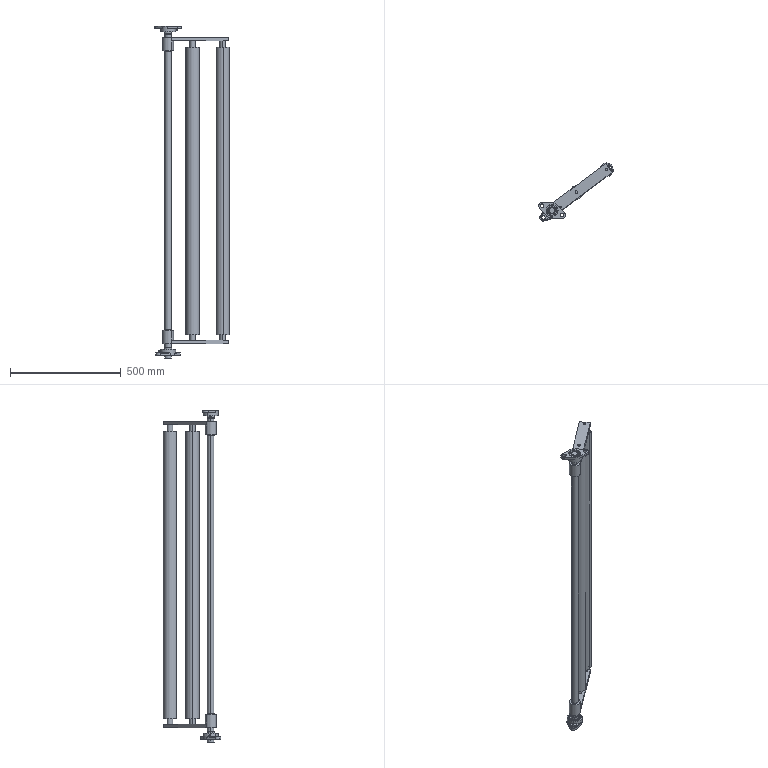Part | SolidWorks | 13 solids | 778 faces | box 336.706 x 259.959 x 1500 mm | volume 5818642 mm3 | torus 248 | cylinder 196 | sphere 136 | plane 126 | spline 42 | cone 30 | commonest cylinder face diameters 2 x24 23 x16 29 x16 30 x14 6.25 x8 12 x8